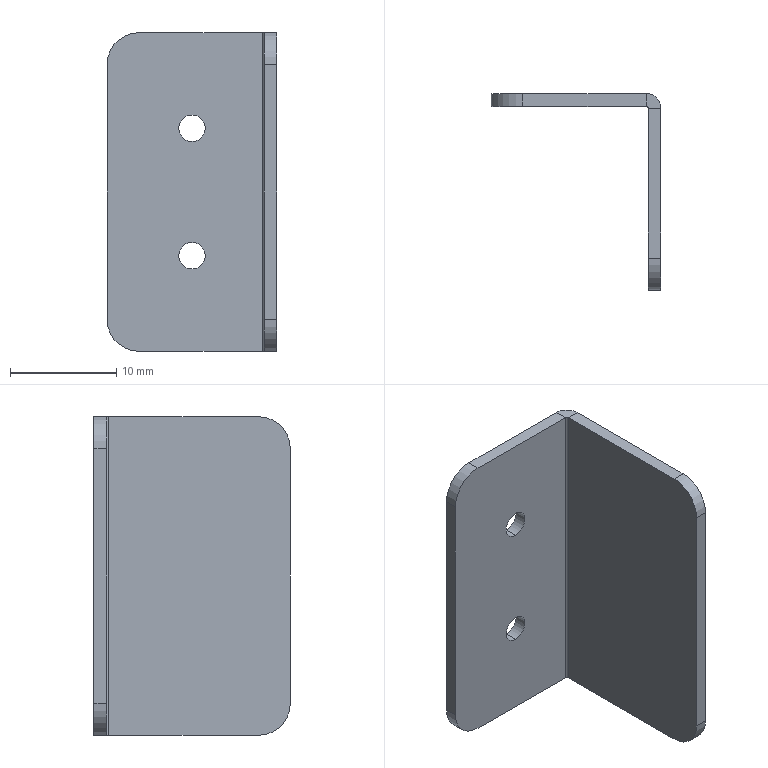Part | SolidWorks | features BaseBody 1 | 1 solid | 22 faces | box 16 x 18.5 x 30 mm | volume 1165 mm3 | plane 12 | cylinder 10 | commonest cylinder face diameters 2.5 x4 6 x4 0.4 x1 2.8 x1
STEP:
#1=CARTESIAN_POINT('',(-8.,-1.2,4.75));
#2=VERTEX_POINT('',#1);
#3=CARTESIAN_POINT('',(-8.,0.,4.75));
#4=VERTEX_POINT('',#3);
#5=CARTESIAN_POINT('',(-8.,0.,4.75));
#6=DIRECTION('',(0.,1.,0.));
#7=VECTOR('',#6,1000.);
#8=LINE('',#5,#7);
#9=EDGE_CURVE('',#2,#4,#8,.T.);
#10=ORIENTED_EDGE('',*,*,#9,.F.);
#11=CARTESIAN_POINT('',(-8.,-1.2,7.25));
#12=VERTEX_POINT('',#11);
#13=CARTESIAN_POINT('',(-8.,-1.2,6.));
#14=DIRECTION('',(0.,1.,0.));
#15=DIRECTION('',(-1.,0.,0.));
#16=AXIS2_PLACEMENT_3D('',#13,#14,#15);
#17=CIRCLE('',#16,1.25);
#18=EDGE_CURVE('',#12,#2,#17,.T.);
#19=ORIENTED_EDGE('',*,*,#18,.F.);
#20=CARTESIAN_POINT('',(-8.,0.,7.25));
#21=VERTEX_POINT('',#20);
#22=CARTESIAN_POINT('',(-8.,0.,7.25));
#23=DIRECTION('',(0.,1.,0.));
#24=VECTOR('',#23,1000.);
#25=LINE('',#22,#24);
#26=EDGE_CURVE('',#12,#21,#25,.T.);
#27=ORIENTED_EDGE('',*,*,#26,.T.);
#28=CARTESIAN_POINT('',(-8.,0.,6.));
#29=DIRECTION('',(0.,1.,0.));
#30=DIRECTION('',(0.,0.,1.));
#31=AXIS2_PLACEMENT_3D('',#28,#29,#30);
#32=CIRCLE('',#31,1.25);
#33=EDGE_CURVE('',#21,#4,#32,.T.);
#34=ORIENTED_EDGE('',*,*,#33,.T.);
#35=EDGE_LOOP('',(#10,#19,#27,#34));
#36=FACE_OUTER_BOUND('',#35,.T.);
#37=CARTESIAN_POINT('',(-8.,0.,6.));
#38=DIRECTION('',(0.,1.,0.));
#39=DIRECTION('',(0.,0.,1.));
#40=AXIS2_PLACEMENT_3D('',#37,#38,#39);
#41=CYLINDRICAL_SURFACE('',#40,1.25);
#42=ADVANCED_FACE('',(#36),#41,.F.);
#43=CARTESIAN_POINT('',(-8.,-1.2,-7.25));
#44=VERTEX_POINT('',#43);
#45=CARTESIAN_POINT('',(-8.,0.,-7.25));
#46=VERTEX_POINT('',#45);
#47=CARTESIAN_POINT('',(-8.,0.,-7.25));
#48=DIRECTION('',(0.,1.,0.));
#49=VECTOR('',#48,1000.);
#50=LINE('',#47,#49);
#51=EDGE_CURVE('',#44,#46,#50,.T.);
#52=ORIENTED_EDGE('',*,*,#51,.F.);
#53=CARTESIAN_POINT('',(-8.,-1.2,-4.75));
#54=VERTEX_POINT('',#53);
#55=CARTESIAN_POINT('',(-8.,-1.2,-6.));
#56=DIRECTION('',(0.,1.,0.));
#57=DIRECTION('',(-1.,0.,0.));
#58=AXIS2_PLACEMENT_3D('',#55,#56,#57);
#59=CIRCLE('',#58,1.25);
#60=EDGE_CURVE('',#54,#44,#59,.T.);
#61=ORIENTED_EDGE('',*,*,#60,.F.);
#62=CARTESIAN_POINT('',(-8.,0.,-4.75));
#63=VERTEX_POINT('',#62);
#64=CARTESIAN_POINT('',(-8.,0.,-4.75));
#65=DIRECTION('',(0.,1.,0.));
#66=VECTOR('',#65,1000.);
#67=LINE('',#64,#66);
#68=EDGE_CURVE('',#54,#63,#67,.T.);
#69=ORIENTED_EDGE('',*,*,#68,.T.);
#70=CARTESIAN_POINT('',(-8.,0.,-6.));
#71=DIRECTION('',(0.,1.,0.));
#72=DIRECTION('',(0.,0.,1.));
#73=AXIS2_PLACEMENT_3D('',#70,#71,#72);
#74=CIRCLE('',#73,1.25);
#75=EDGE_CURVE('',#63,#46,#74,.T.);
#76=ORIENTED_EDGE('',*,*,#75,.T.);
#77=EDGE_LOOP('',(#52,#61,#69,#76));
#78=FACE_OUTER_BOUND('',#77,.T.);
#79=CARTESIAN_POINT('',(-8.,0.,-6.));
#80=DIRECTION('',(0.,1.,0.));
#81=DIRECTION('',(0.,0.,1.));
#82=AXIS2_PLACEMENT_3D('',#79,#80,#81);
#83=CYLINDRICAL_SURFACE('',#82,1.25);
#84=ADVANCED_FACE('',(#78),#83,.F.);
#85=CARTESIAN_POINT('',(0.,-15.5,15.));
#86=VERTEX_POINT('',#85);
#87=CARTESIAN_POINT('',(0.,-18.5,12.));
#88=VERTEX_POINT('',#87);
#89=CARTESIAN_POINT('',(0.,-15.5,12.));
#90=DIRECTION('',(1.,0.,0.));
#91=DIRECTION('',(0.,1.,0.));
#92=AXIS2_PLACEMENT_3D('',#89,#90,#91);
#93=CIRCLE('',#92,3.);
#94=EDGE_CURVE('',#86,#88,#93,.T.);
#95=ORIENTED_EDGE('',*,*,#94,.F.);
#96=CARTESIAN_POINT('',(-1.2,-15.5,15.));
#97=VERTEX_POINT('',#96);
#98=CARTESIAN_POINT('',(-1.4,-15.5,15.));
#99=DIRECTION('',(1.,0.,0.));
#100=VECTOR('',#99,1000.);
#101=LINE('',#98,#100);
#102=EDGE_CURVE('',#97,#86,#101,.T.);
#103=ORIENTED_EDGE('',*,*,#102,.F.);
#104=CARTESIAN_POINT('',(-1.2,-18.5,12.));
#105=VERTEX_POINT('',#104);
#106=CARTESIAN_POINT('',(-1.2,-15.5,12.));
#107=DIRECTION('',(-1.,0.,0.));
#108=DIRECTION('',(0.,1.,0.));
#109=AXIS2_PLACEMENT_3D('',#106,#107,#108);
#110=CIRCLE('',#109,3.);
#111=EDGE_CURVE('',#105,#97,#110,.T.);
#112=ORIENTED_EDGE('',*,*,#111,.F.);
#113=CARTESIAN_POINT('',(0.,-18.5,12.));
#114=DIRECTION('',(-1.,0.,0.));
#115=VECTOR('',#114,1000.);
#116=LINE('',#113,#115);
#117=EDGE_CURVE('',#88,#105,#116,.T.);
#118=ORIENTED_EDGE('',*,*,#117,.F.);
#119=EDGE_LOOP('',(#95,#103,#112,#118));
#120=FACE_OUTER_BOUND('',#119,.T.);
#121=CARTESIAN_POINT('',(0.,-15.5,12.));
#122=DIRECTION('',(-1.,0.,0.));
#123=DIRECTION('',(0.,0.,1.));
#124=AXIS2_PLACEMENT_3D('',#121,#122,#123);
#125=CYLINDRICAL_SURFACE('',#124,3.);
#126=ADVANCED_FACE('',(#120),#125,.T.);
#127=CARTESIAN_POINT('',(0.,-18.5,-12.));
#128=VERTEX_POINT('',#127);
#129=CARTESIAN_POINT('',(0.,-15.5,-15.));
#130=VERTEX_POINT('',#129);
#131=CARTESIAN_POINT('',(0.,-15.5,-12.));
#132=DIRECTION('',(1.,0.,0.));
#133=DIRECTION('',(0.,1.,0.));
#134=AXIS2_PLACEMENT_3D('',#131,#132,#133);
#135=CIRCLE('',#134,3.);
#136=EDGE_CURVE('',#128,#130,#135,.T.);
#137=ORIENTED_EDGE('',*,*,#136,.F.);
#138=CARTESIAN_POINT('',(-1.2,-18.5,-12.));
#139=VERTEX_POINT('',#138);
#140=CARTESIAN_POINT('',(0.,-18.5,-12.));
#141=DIRECTION('',(1.,0.,0.));
#142=VECTOR('',#141,1000.);
#143=LINE('',#140,#142);
#144=EDGE_CURVE('',#139,#128,#143,.T.);
#145=ORIENTED_EDGE('',*,*,#144,.F.);
#146=CARTESIAN_POINT('',(-1.2,-15.5,-15.));
#147=VERTEX_POINT('',#146);
#148=CARTESIAN_POINT('',(-1.2,-15.5,-12.));
#149=DIRECTION('',(-1.,0.,0.));
#150=DIRECTION('',(0.,1.,0.));
#151=AXIS2_PLACEMENT_3D('',#148,#149,#150);
#152=CIRCLE('',#151,3.);
#153=EDGE_CURVE('',#147,#139,#152,.T.);
#154=ORIENTED_EDGE('',*,*,#153,.F.);
#155=CARTESIAN_POINT('',(-1.2,-15.5,-15.));
#156=DIRECTION('',(-1.,0.,0.));
#157=VECTOR('',#156,1000.);
#158=LINE('',#155,#157);
#159=EDGE_CURVE('',#130,#147,#158,.T.);
#160=ORIENTED_EDGE('',*,*,#159,.F.);
#161=EDGE_LOOP('',(#137,#145,#154,#160));
#162=FACE_OUTER_BOUND('',#161,.T.);
#163=CARTESIAN_POINT('',(-1.4,-15.5,-12.));
#164=DIRECTION('',(1.,0.,0.));
#165=DIRECTION('',(0.,0.,-1.));
#166=AXIS2_PLACEMENT_3D('',#163,#164,#165);
#167=CYLINDRICAL_SURFACE('',#166,3.);
#168=ADVANCED_FACE('',(#162),#167,.T.);
#169=CARTESIAN_POINT('',(-16.,-1.2,-12.));
#170=VERTEX_POINT('',#169);
#171=CARTESIAN_POINT('',(-13.,-1.2,-15.));
#172=VERTEX_POINT('',#171);
#173=CARTESIAN_POINT('',(-13.,-1.2,-12.));
#174=DIRECTION('',(0.,-1.,0.));
#175=DIRECTION('',(-1.,0.,0.));
#176=AXIS2_PLACEMENT_3D('',#173,#174,#175);
#177=CIRCLE('',#176,3.);
#178=EDGE_CURVE('',#170,#172,#177,.T.);
#179=ORIENTED_EDGE('',*,*,#178,.F.);
#180=CARTESIAN_POINT('',(-16.,0.,-12.));
#181=VERTEX_POINT('',#180);
#182=CARTESIAN_POINT('',(-16.,-1.2,-12.));
#183=DIRECTION('',(0.,-1.,0.));
#184=VECTOR('',#183,1000.);
#185=LINE('',#182,#184);
#186=EDGE_CURVE('',#181,#170,#185,.T.);
#187=ORIENTED_EDGE('',*,*,#186,.F.);
#188=CARTESIAN_POINT('',(-13.,0.,-15.));
#189=VERTEX_POINT('',#188);
#190=CARTESIAN_POINT('',(-13.,0.,-12.));
#191=DIRECTION('',(0.,1.,0.));
#192=DIRECTION('',(-1.,0.,0.));
#193=AXIS2_PLACEMENT_3D('',#190,#191,#192);
#194=CIRCLE('',#193,3.);
#195=EDGE_CURVE('',#189,#181,#194,.T.);
#196=ORIENTED_EDGE('',*,*,#195,.F.);
#197=CARTESIAN_POINT('',(-13.,-1.4,-15.));
#198=DIRECTION('',(0.,1.,0.));
#199=VECTOR('',#198,1000.);
#200=LINE('',#197,#199);
#201=EDGE_CURVE('',#172,#189,#200,.T.);
#202=ORIENTED_EDGE('',*,*,#201,.F.);
#203=EDGE_LOOP('',(#179,#187,#196,#202));
#204=FACE_OUTER_BOUND('',#203,.T.);
#205=CARTESIAN_POINT('',(-13.,-1.4,-12.));
#206=DIRECTION('',(0.,1.,0.));
#207=DIRECTION('',(0.,0.,1.));
#208=AXIS2_PLACEMENT_3D('',#205,#206,#207);
#209=CYLINDRICAL_SURFACE('',#208,3.);
#210=ADVANCED_FACE('',(#204),#209,.T.);
#211=CARTESIAN_POINT('',(-13.,-1.2,15.));
#212=VERTEX_POINT('',#211);
#213=CARTESIAN_POINT('',(-16.,-1.2,12.));
#214=VERTEX_POINT('',#213);
#215=CARTESIAN_POINT('',(-13.,-1.2,12.));
#216=DIRECTION('',(0.,-1.,0.));
#217=DIRECTION('',(-1.,0.,0.));
#218=AXIS2_PLACEMENT_3D('',#215,#216,#217);
#219=CIRCLE('',#218,3.);
#220=EDGE_CURVE('',#212,#214,#219,.T.);
#221=ORIENTED_EDGE('',*,*,#220,.F.);
#222=CARTESIAN_POINT('',(-13.,0.,15.));
#223=VERTEX_POINT('',#222);
#224=CARTESIAN_POINT('',(-13.,-1.4,15.));
#225=DIRECTION('',(0.,-1.,0.));
#226=VECTOR('',#225,1000.);
#227=LINE('',#224,#226);
#228=EDGE_CURVE('',#223,#212,#227,.T.);
#229=ORIENTED_EDGE('',*,*,#228,.F.);
#230=CARTESIAN_POINT('',(-16.,0.,12.));
#231=VERTEX_POINT('',#230);
#232=CARTESIAN_POINT('',(-13.,0.,12.));
#233=DIRECTION('',(0.,1.,0.));
#234=DIRECTION('',(-1.,0.,0.));
#235=AXIS2_PLACEMENT_3D('',#232,#233,#234);
#236=CIRCLE('',#235,3.);
#237=EDGE_CURVE('',#231,#223,#236,.T.);
#238=ORIENTED_EDGE('',*,*,#237,.F.);
#239=CARTESIAN_POINT('',(-16.,-1.2,12.));
#240=DIRECTION('',(0.,1.,0.));
#241=VECTOR('',#240,1000.);
#242=LINE('',#239,#241);
#243=EDGE_CURVE('',#214,#231,#242,.T.);
#244=ORIENTED_EDGE('',*,*,#243,.F.);
#245=EDGE_LOOP('',(#221,#229,#238,#244));
#246=FACE_OUTER_BOUND('',#245,.T.);
#247=CARTESIAN_POINT('',(-13.,-1.2,12.));
#248=DIRECTION('',(0.,1.,0.));
#249=DIRECTION('',(0.,0.,1.));
#250=AXIS2_PLACEMENT_3D('',#247,#248,#249);
#251=CYLINDRICAL_SURFACE('',#250,3.);
#252=ADVANCED_FACE('',(#246),#251,.T.);
#253=CARTESIAN_POINT('',(0.,-1.4,-15.));
#254=VERTEX_POINT('',#253);
#255=CARTESIAN_POINT('',(0.,0.,-15.));
#256=DIRECTION('',(0.,-1.,0.));
#257=VECTOR('',#256,1000.);
#258=LINE('',#255,#257);
#259=EDGE_CURVE('',#254,#130,#258,.T.);
#260=ORIENTED_EDGE('',*,*,#259,.T.);
#261=ORIENTED_EDGE('',*,*,#159,.T.);
#262=CARTESIAN_POINT('',(-1.2,-1.4,-15.));
#263=VERTEX_POINT('',#262);
#264=CARTESIAN_POINT('',(-1.2,0.,-15.));
#265=DIRECTION('',(0.,-1.,0.));
#266=VECTOR('',#265,1000.);
#267=LINE('',#264,#266);
#268=EDGE_CURVE('',#263,#147,#267,.T.);
#269=ORIENTED_EDGE('',*,*,#268,.F.);
#270=CARTESIAN_POINT('',(-1.2,-1.4,-15.));
#271=DIRECTION('',(1.,0.,0.));
#272=VECTOR('',#271,1000.);
#273=LINE('',#270,#272);
#274=EDGE_CURVE('',#263,#254,#273,.T.);
#275=ORIENTED_EDGE('',*,*,#274,.T.);
#276=EDGE_LOOP('',(#260,#261,#269,#275));
#277=FACE_OUTER_BOUND('',#276,.T.);
#278=CARTESIAN_POINT('',(-1.4,-1.4,-15.));
#279=DIRECTION('',(0.,0.,1.));
#280=DIRECTION('',(1.,0.,0.));
#281=AXIS2_PLACEMENT_3D('',#278,#279,#280);
#282=PLANE('',#281);
#283=ADVANCED_FACE('',(#277),#282,.F.);
#284=CARTESIAN_POINT('',(-1.4,0.,15.));
#285=VERTEX_POINT('',#284);
#286=CARTESIAN_POINT('',(0.,0.,15.));
#287=DIRECTION('',(1.,0.,0.));
#288=VECTOR('',#287,1000.);
#289=LINE('',#286,#288);
#290=EDGE_CURVE('',#223,#285,#289,.T.);
#291=ORIENTED_EDGE('',*,*,#290,.F.);
#292=ORIENTED_EDGE('',*,*,#228,.T.);
#293=CARTESIAN_POINT('',(-1.4,-1.2,15.));
#294=VERTEX_POINT('',#293);
#295=CARTESIAN_POINT('',(0.,-1.2,15.));
#296=DIRECTION('',(1.,0.,0.));
#297=VECTOR('',#296,1000.);
#298=LINE('',#295,#297);
#299=EDGE_CURVE('',#212,#294,#298,.T.);
#300=ORIENTED_EDGE('',*,*,#299,.T.);
#301=CARTESIAN_POINT('',(-1.4,-1.2,15.));
#302=DIRECTION('',(0.,1.,0.));
#303=VECTOR('',#302,1000.);
#304=LINE('',#301,#303);
#305=EDGE_CURVE('',#294,#285,#304,.T.);
#306=ORIENTED_EDGE('',*,*,#305,.T.);
#307=EDGE_LOOP('',(#291,#292,#300,#306));
#308=FACE_OUTER_BOUND('',#307,.T.);
#309=CARTESIAN_POINT('',(-1.4,-1.4,15.));
#310=DIRECTION('',(0.,0.,1.));
#311=DIRECTION('',(1.,0.,0.));
#312=AXIS2_PLACEMENT_3D('',#309,#310,#311);
#313=PLANE('',#312);
#314=ADVANCED_FACE('',(#308),#313,.T.);
#315=CARTESIAN_POINT('',(-1.4,-1.2,-15.));
#316=VERTEX_POINT('',#315);
#317=CARTESIAN_POINT('',(-1.4,-1.4,-15.));
#318=DIRECTION('',(0.,0.,-1.));
#319=DIRECTION('',(1.,0.,0.));
#320=AXIS2_PLACEMENT_3D('',#317,#318,#319);
#321=CIRCLE('',#320,0.2);
#322=EDGE_CURVE('',#316,#263,#321,.T.);
#323=ORIENTED_EDGE('',*,*,#322,.T.);
#324=CARTESIAN_POINT('',(-1.2,-1.4,15.));
#325=VERTEX_POINT('',#324);
#326=CARTESIAN_POINT('',(-1.2,-1.4,15.));
#327=DIRECTION('',(0.,0.,-1.));
#328=VECTOR('',#327,1000.);
#329=LINE('',#326,#328);
#330=EDGE_CURVE('',#325,#263,#329,.T.);
#331=ORIENTED_EDGE('',*,*,#330,.F.);
#332=CARTESIAN_POINT('',(-1.4,-1.4,15.));
#333=DIRECTION('',(0.,0.,-1.));
#334=DIRECTION('',(1.,0.,0.));
#335=AXIS2_PLACEMENT_3D('',#332,#333,#334);
#336=CIRCLE('',#335,0.2);
#337=EDGE_CURVE('',#294,#325,#336,.T.);
#338=ORIENTED_EDGE('',*,*,#337,.F.);
#339=CARTESIAN_POINT('',(-1.4,-1.2,15.));
#340=DIRECTION('',(0.,0.,-1.));
#341=VECTOR('',#340,1000.);
#342=LINE('',#339,#341);
#343=EDGE_CURVE('',#294,#316,#342,.T.);
#344=ORIENTED_EDGE('',*,*,#343,.T.);
#345=EDGE_LOOP('',(#323,#331,#338,#344));
#346=FACE_OUTER_BOUND('',#345,.T.);
#347=CARTESIAN_POINT('',(-1.4,-1.4,15.));
#348=DIRECTION('',(0.,0.,-1.));
#349=DIRECTION('',(-1.,0.,0.));
#350=AXIS2_PLACEMENT_3D('',#347,#348,#349);
#351=CYLINDRICAL_SURFACE('',#350,0.2);
#352=ADVANCED_FACE('',(#346),#351,.F.);
#353=ORIENTED_EDGE('',*,*,#60,.T.);
#354=CARTESIAN_POINT('',(-8.,-1.2,-6.));
#355=DIRECTION('',(0.,1.,0.));
#356=DIRECTION('',(-1.,0.,0.));
#357=AXIS2_PLACEMENT_3D('',#354,#355,#356);
#358=CIRCLE('',#357,1.25);
#359=EDGE_CURVE('',#44,#54,#358,.T.);
#360=ORIENTED_EDGE('',*,*,#359,.T.);
#361=EDGE_LOOP('',(#353,#360));
#362=FACE_BOUND('',#361,.T.);
#363=ORIENTED_EDGE('',*,*,#18,.T.);
#364=CARTESIAN_POINT('',(-8.,-1.2,6.));
#365=DIRECTION('',(0.,1.,0.));
#366=DIRECTION('',(-1.,0.,0.));
#367=AXIS2_PLACEMENT_3D('',#364,#365,#366);
#368=CIRCLE('',#367,1.25);
#369=EDGE_CURVE('',#2,#12,#368,.T.);
#370=ORIENTED_EDGE('',*,*,#369,.T.);
#371=EDGE_LOOP('',(#363,#370));
#372=FACE_BOUND('',#371,.T.);
#373=ORIENTED_EDGE('',*,*,#299,.F.);
#374=ORIENTED_EDGE('',*,*,#220,.T.);
#375=CARTESIAN_POINT('',(-16.,-1.2,15.));
#376=DIRECTION('',(0.,0.,-1.));
#377=VECTOR('',#376,1000.);
#378=LINE('',#375,#377);
#379=EDGE_CURVE('',#214,#170,#378,.T.);
#380=ORIENTED_EDGE('',*,*,#379,.T.);
#381=ORIENTED_EDGE('',*,*,#178,.T.);
#382=CARTESIAN_POINT('',(0.,-1.2,-15.));
#383=DIRECTION('',(1.,0.,0.));
#384=VECTOR('',#383,1000.);
#385=LINE('',#382,#384);
#386=EDGE_CURVE('',#172,#316,#385,.T.);
#387=ORIENTED_EDGE('',*,*,#386,.T.);
#388=ORIENTED_EDGE('',*,*,#343,.F.);
#389=EDGE_LOOP('',(#373,#374,#380,#381,#387,#388));
#390=FACE_OUTER_BOUND('',#389,.T.);
#391=CARTESIAN_POINT('',(0.,-1.2,15.));
#392=DIRECTION('',(0.,1.,0.));
#393=DIRECTION('',(1.,0.,0.));
#394=AXIS2_PLACEMENT_3D('',#391,#392,#393);
#395=PLANE('',#394);
#396=ADVANCED_FACE('',(#362,#372,#390),#395,.F.);
#397=ORIENTED_EDGE('',*,*,#379,.F.);
#398=ORIENTED_EDGE('',*,*,#243,.T.);
#399=CARTESIAN_POINT('',(-16.,0.,15.));
#400=DIRECTION('',(0.,0.,-1.));
#401=VECTOR('',#400,1000.);
#402=LINE('',#399,#401);
#403=EDGE_CURVE('',#231,#181,#402,.T.);
#404=ORIENTED_EDGE('',*,*,#403,.T.);
#405=ORIENTED_EDGE('',*,*,#186,.T.);
#406=EDGE_LOOP('',(#397,#398,#404,#405));
#407=FACE_OUTER_BOUND('',#406,.T.);
#408=CARTESIAN_POINT('',(-16.,-1.2,15.));
#409=DIRECTION('',(-1.,0.,0.));
#410=DIRECTION('',(0.,0.,1.));
#411=AXIS2_PLACEMENT_3D('',#408,#409,#410);
#412=PLANE('',#411);
#413=ADVANCED_FACE('',(#407),#412,.T.);
#414=ORIENTED_EDGE('',*,*,#75,.F.);
#415=CARTESIAN_POINT('',(-8.,0.,-6.));
#416=DIRECTION('',(0.,1.,0.));
#417=DIRECTION('',(0.,0.,1.));
#418=AXIS2_PLACEMENT_3D('',#415,#416,#417);
#419=CIRCLE('',#418,1.25);
#420=EDGE_CURVE('',#46,#63,#419,.T.);
#421=ORIENTED_EDGE('',*,*,#420,.F.);
#422=EDGE_LOOP('',(#414,#421));
#423=FACE_BOUND('',#422,.T.);
#424=ORIENTED_EDGE('',*,*,#33,.F.);
#425=CARTESIAN_POINT('',(-8.,0.,6.));
#426=DIRECTION('',(0.,1.,0.));
#427=DIRECTION('',(0.,0.,1.));
#428=AXIS2_PLACEMENT_3D('',#425,#426,#427);
#429=CIRCLE('',#428,1.25);
#430=EDGE_CURVE('',#4,#21,#429,.T.);
#431=ORIENTED_EDGE('',*,*,#430,.F.);
#432=EDGE_LOOP('',(#424,#431));
#433=FACE_BOUND('',#432,.T.);
#434=ORIENTED_EDGE('',*,*,#403,.F.);
#435=ORIENTED_EDGE('',*,*,#237,.T.);
#436=ORIENTED_EDGE('',*,*,#290,.T.);
#437=CARTESIAN_POINT('',(-1.4,0.,-15.));
#438=VERTEX_POINT('',#437);
#439=CARTESIAN_POINT('',(-1.4,0.,15.));
#440=DIRECTION('',(0.,0.,-1.));
#441=VECTOR('',#440,1000.);
#442=LINE('',#439,#441);
#443=EDGE_CURVE('',#285,#438,#442,.T.);
#444=ORIENTED_EDGE('',*,*,#443,.T.);
#445=CARTESIAN_POINT('',(0.,0.,-15.));
#446=DIRECTION('',(1.,0.,0.));
#447=VECTOR('',#446,1000.);
#448=LINE('',#445,#447);
#449=EDGE_CURVE('',#189,#438,#448,.T.);
#450=ORIENTED_EDGE('',*,*,#449,.F.);
#451=ORIENTED_EDGE('',*,*,#195,.T.);
#452=EDGE_LOOP('',(#434,#435,#436,#444,#450,#451));
#453=FACE_OUTER_BOUND('',#452,.T.);
#454=CARTESIAN_POINT('',(0.,0.,15.));
#455=DIRECTION('',(0.,1.,0.));
#456=DIRECTION('',(1.,0.,0.));
#457=AXIS2_PLACEMENT_3D('',#454,#455,#456);
#458=PLANE('',#457);
#459=ADVANCED_FACE('',(#423,#433,#453),#458,.T.);
#460=CARTESIAN_POINT('',(-1.4,-1.4,-15.));
#461=DIRECTION('',(0.,0.,-1.));
#462=DIRECTION('',(1.,0.,0.));
#463=AXIS2_PLACEMENT_3D('',#460,#461,#462);
#464=CIRCLE('',#463,1.4);
#465=EDGE_CURVE('',#438,#254,#464,.T.);
#466=ORIENTED_EDGE('',*,*,#465,.F.);
#467=ORIENTED_EDGE('',*,*,#443,.F.);
#468=CARTESIAN_POINT('',(0.,-1.4,15.));
#469=VERTEX_POINT('',#468);
#470=CARTESIAN_POINT('',(-1.4,-1.4,15.));
#471=DIRECTION('',(0.,0.,-1.));
#472=DIRECTION('',(1.,0.,0.));
#473=AXIS2_PLACEMENT_3D('',#470,#471,#472);
#474=CIRCLE('',#473,1.4);
#475=EDGE_CURVE('',#285,#469,#474,.T.);
#476=ORIENTED_EDGE('',*,*,#475,.T.);
#477=CARTESIAN_POINT('',(0.,-1.4,15.));
#478=DIRECTION('',(0.,0.,-1.));
#479=VECTOR('',#478,1000.);
#480=LINE('',#477,#479);
#481=EDGE_CURVE('',#469,#254,#480,.T.);
#482=ORIENTED_EDGE('',*,*,#481,.T.);
#483=EDGE_LOOP('',(#466,#467,#476,#482));
#484=FACE_OUTER_BOUND('',#483,.T.);
#485=CARTESIAN_POINT('',(-1.4,-1.4,15.));
#486=DIRECTION('',(0.,0.,-1.));
#487=DIRECTION('',(-1.,0.,0.));
#488=AXIS2_PLACEMENT_3D('',#485,#486,#487);
#489=CYLINDRICAL_SURFACE('',#488,1.4);
#490=ADVANCED_FACE('',(#484),#489,.T.);
#491=CARTESIAN_POINT('',(0.,-18.5,15.));
#492=DIRECTION('',(0.,0.,-1.));
#493=VECTOR('',#492,1000.);
#494=LINE('',#491,#493);
#495=EDGE_CURVE('',#88,#128,#494,.T.);
#496=ORIENTED_EDGE('',*,*,#495,.T.);
#497=ORIENTED_EDGE('',*,*,#136,.T.);
#498=ORIENTED_EDGE('',*,*,#259,.F.);
#499=ORIENTED_EDGE('',*,*,#481,.F.);
#500=CARTESIAN_POINT('',(0.,0.,15.));
#501=DIRECTION('',(0.,-1.,0.));
#502=VECTOR('',#501,1000.);
#503=LINE('',#500,#502);
#504=EDGE_CURVE('',#469,#86,#503,.T.);
#505=ORIENTED_EDGE('',*,*,#504,.T.);
#506=ORIENTED_EDGE('',*,*,#94,.T.);
#507=EDGE_LOOP('',(#496,#497,#498,#499,#505,#506));
#508=FACE_OUTER_BOUND('',#507,.T.);
#509=CARTESIAN_POINT('',(0.,0.,15.));
#510=DIRECTION('',(1.,0.,0.));
#511=DIRECTION('',(0.,1.,0.));
#512=AXIS2_PLACEMENT_3D('',#509,#510,#511);
#513=PLANE('',#512);
#514=ADVANCED_FACE('',(#508),#513,.T.);
#515=CARTESIAN_POINT('',(-1.2,-18.5,15.));
#516=DIRECTION('',(0.,0.,-1.));
#517=VECTOR('',#516,1000.);
#518=LINE('',#515,#517);
#519=EDGE_CURVE('',#105,#139,#518,.T.);
#520=ORIENTED_EDGE('',*,*,#519,.T.);
#521=ORIENTED_EDGE('',*,*,#144,.T.);
#522=ORIENTED_EDGE('',*,*,#495,.F.);
#523=ORIENTED_EDGE('',*,*,#117,.T.);
#524=EDGE_LOOP('',(#520,#521,#522,#523));
#525=FACE_OUTER_BOUND('',#524,.T.);
#526=CARTESIAN_POINT('',(0.,-18.5,15.));
#527=DIRECTION('',(0.,-1.,0.));
#528=DIRECTION('',(0.,0.,-1.));
#529=AXIS2_PLACEMENT_3D('',#526,#527,#528);
#530=PLANE('',#529);
#531=ADVANCED_FACE('',(#525),#530,.T.);
#532=ORIENTED_EDGE('',*,*,#268,.T.);
#533=ORIENTED_EDGE('',*,*,#153,.T.);
#534=ORIENTED_EDGE('',*,*,#519,.F.);
#535=ORIENTED_EDGE('',*,*,#111,.T.);
#536=CARTESIAN_POINT('',(-1.2,0.,15.));
#537=DIRECTION('',(0.,-1.,0.));
#538=VECTOR('',#537,1000.);
#539=LINE('',#536,#538);
#540=EDGE_CURVE('',#325,#97,#539,.T.);
#541=ORIENTED_EDGE('',*,*,#540,.F.);
#542=ORIENTED_EDGE('',*,*,#330,.T.);
#543=EDGE_LOOP('',(#532,#533,#534,#535,#541,#542));
#544=FACE_OUTER_BOUND('',#543,.T.);
#545=CARTESIAN_POINT('',(-1.2,0.,15.));
#546=DIRECTION('',(1.,0.,0.));
#547=DIRECTION('',(0.,1.,0.));
#548=AXIS2_PLACEMENT_3D('',#545,#546,#547);
#549=PLANE('',#548);
#550=ADVANCED_FACE('',(#544),#549,.F.);
#551=ORIENTED_EDGE('',*,*,#386,.F.);
#552=ORIENTED_EDGE('',*,*,#201,.T.);
#553=ORIENTED_EDGE('',*,*,#449,.T.);
#554=CARTESIAN_POINT('',(-1.4,0.,-15.));
#555=DIRECTION('',(0.,-1.,0.));
#556=VECTOR('',#555,1000.);
#557=LINE('',#554,#556);
#558=EDGE_CURVE('',#438,#316,#557,.T.);
#559=ORIENTED_EDGE('',*,*,#558,.T.);
#560=EDGE_LOOP('',(#551,#552,#553,#559));
#561=FACE_OUTER_BOUND('',#560,.T.);
#562=CARTESIAN_POINT('',(-1.2,-1.4,-15.));
#563=DIRECTION('',(0.,0.,-1.));
#564=DIRECTION('',(0.,-1.,0.));
#565=AXIS2_PLACEMENT_3D('',#562,#563,#564);
#566=PLANE('',#565);
#567=ADVANCED_FACE('',(#561),#566,.T.);
#568=ORIENTED_EDGE('',*,*,#558,.F.);
#569=ORIENTED_EDGE('',*,*,#465,.T.);
#570=ORIENTED_EDGE('',*,*,#274,.F.);
#571=ORIENTED_EDGE('',*,*,#322,.F.);
#572=EDGE_LOOP('',(#568,#569,#570,#571));
#573=FACE_OUTER_BOUND('',#572,.T.);
#574=CARTESIAN_POINT('',(-1.4,0.,-15.));
#575=DIRECTION('',(0.,0.,-1.));
#576=DIRECTION('',(0.,-1.,0.));
#577=AXIS2_PLACEMENT_3D('',#574,#575,#576);
#578=PLANE('',#577);
#579=ADVANCED_FACE('',(#573),#578,.T.);
#580=ORIENTED_EDGE('',*,*,#540,.T.);
#581=ORIENTED_EDGE('',*,*,#102,.T.);
#582=ORIENTED_EDGE('',*,*,#504,.F.);
#583=CARTESIAN_POINT('',(0.,-1.4,15.));
#584=DIRECTION('',(-1.,0.,0.));
#585=VECTOR('',#584,1000.);
#586=LINE('',#583,#585);
#587=EDGE_CURVE('',#469,#325,#586,.T.);
#588=ORIENTED_EDGE('',*,*,#587,.T.);
#589=EDGE_LOOP('',(#580,#581,#582,#588));
#590=FACE_OUTER_BOUND('',#589,.T.);
#591=CARTESIAN_POINT('',(-1.4,-1.2,15.));
#592=DIRECTION('',(0.,0.,1.));
#593=DIRECTION('',(1.,0.,0.));
#594=AXIS2_PLACEMENT_3D('',#591,#592,#593);
#595=PLANE('',#594);
#596=ADVANCED_FACE('',(#590),#595,.T.);
#597=ORIENTED_EDGE('',*,*,#587,.F.);
#598=ORIENTED_EDGE('',*,*,#475,.F.);
#599=ORIENTED_EDGE('',*,*,#305,.F.);
#600=ORIENTED_EDGE('',*,*,#337,.T.);
#601=EDGE_LOOP('',(#597,#598,#599,#600));
#602=FACE_OUTER_BOUND('',#601,.T.);
#603=CARTESIAN_POINT('',(0.,-1.4,15.));
#604=DIRECTION('',(0.,0.,1.));
#605=DIRECTION('',(1.,0.,0.));
#606=AXIS2_PLACEMENT_3D('',#603,#604,#605);
#607=PLANE('',#606);
#608=ADVANCED_FACE('',(#602),#607,.T.);
#609=ORIENTED_EDGE('',*,*,#359,.F.);
#610=ORIENTED_EDGE('',*,*,#51,.T.);
#611=ORIENTED_EDGE('',*,*,#420,.T.);
#612=ORIENTED_EDGE('',*,*,#68,.F.);
#613=EDGE_LOOP('',(#609,#610,#611,#612));
#614=FACE_OUTER_BOUND('',#613,.T.);
#615=CARTESIAN_POINT('',(-8.,0.,-6.));
#616=DIRECTION('',(0.,1.,0.));
#617=DIRECTION('',(0.,0.,1.));
#618=AXIS2_PLACEMENT_3D('',#615,#616,#617);
#619=CYLINDRICAL_SURFACE('',#618,1.25);
#620=ADVANCED_FACE('',(#614),#619,.F.);
#621=ORIENTED_EDGE('',*,*,#369,.F.);
#622=ORIENTED_EDGE('',*,*,#9,.T.);
#623=ORIENTED_EDGE('',*,*,#430,.T.);
#624=ORIENTED_EDGE('',*,*,#26,.F.);
#625=EDGE_LOOP('',(#621,#622,#623,#624));
#626=FACE_OUTER_BOUND('',#625,.T.);
#627=CARTESIAN_POINT('',(-8.,0.,6.));
#628=DIRECTION('',(0.,1.,0.));
#629=DIRECTION('',(0.,0.,1.));
#630=AXIS2_PLACEMENT_3D('',#627,#628,#629);
#631=CYLINDRICAL_SURFACE('',#630,1.25);
#632=ADVANCED_FACE('',(#626),#631,.F.);
#633=CLOSED_SHELL('',(#42,#84,#126,#168,#210,#252,#283,#314,#352,#396,#413,#459,#490,#514,#531,#550,#567,#579,#596,#608,#620,#632));
#634=MANIFOLD_SOLID_BREP('',#633);
#635=CARTESIAN_POINT('',(0.,0.,0.));
#636=DIRECTION('',(0.,0.,1.));
#637=DIRECTION('',(1.,0.,0.));
#638=AXIS2_PLACEMENT_3D('',#635,#636,#637);
#639=(LENGTH_UNIT()NAMED_UNIT(*)SI_UNIT(.MILLI.,.METRE.));
#640=UNCERTAINTY_MEASURE_WITH_UNIT(LENGTH_MEASURE(0.00001),#639,'','');
#641=(NAMED_UNIT(*)PLANE_ANGLE_UNIT()SI_UNIT($,.RADIAN.));
#642=(NAMED_UNIT(*)SI_UNIT($,.STERADIAN.)SOLID_ANGLE_UNIT());
#643=(GEOMETRIC_REPRESENTATION_CONTEXT(3)GLOBAL_UNCERTAINTY_ASSIGNED_CONTEXT((#640))GLOBAL_UNIT_ASSIGNED_CONTEXT((#639,#641,#642))REPRESENTATION_CONTEXT('',''));
#644=ADVANCED_BREP_SHAPE_REPRESENTATION('',(#634,#638),#643);